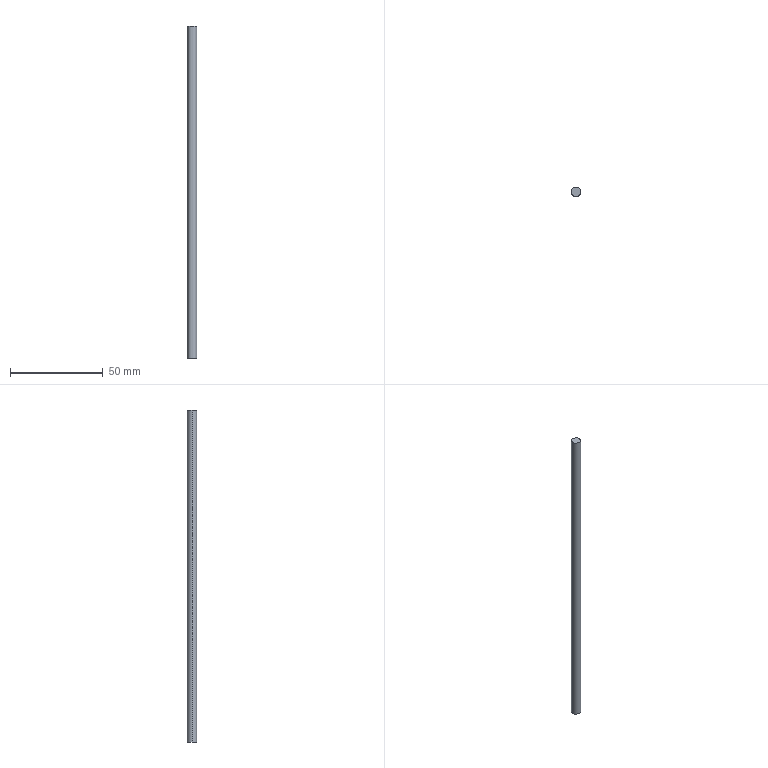Part | SolidWorks | features Extrusion 1 | 1 solid | 4 faces | box 5 x 5 x 178.5 mm | volume 3505 mm3 | cylinder 2 | plane 2 | commonest cylinder face diameters 5 x2
STEP:
#1=CARTESIAN_POINT('',(2.5,0.,178.5));
#2=VERTEX_POINT('',#1);
#3=CARTESIAN_POINT('',(-2.5,0.,178.5));
#4=VERTEX_POINT('',#3);
#5=CARTESIAN_POINT('',(0.,0.,178.5));
#6=DIRECTION('',(0.,0.,1.));
#7=DIRECTION('',(1.,0.,0.));
#8=AXIS2_PLACEMENT_3D('',#5,#6,#7);
#9=CIRCLE('',#8,2.5);
#10=EDGE_CURVE('',#2,#4,#9,.T.);
#11=ORIENTED_EDGE('',*,*,#10,.F.);
#12=CARTESIAN_POINT('',(2.5,0.,0.));
#13=VERTEX_POINT('',#12);
#14=CARTESIAN_POINT('',(2.5,0.,178.5));
#15=DIRECTION('',(0.,0.,-1.));
#16=VECTOR('',#15,1000.);
#17=LINE('',#14,#16);
#18=EDGE_CURVE('',#2,#13,#17,.T.);
#19=ORIENTED_EDGE('',*,*,#18,.T.);
#20=CARTESIAN_POINT('',(-2.5,0.,0.));
#21=VERTEX_POINT('',#20);
#22=CARTESIAN_POINT('',(0.,0.,0.));
#23=DIRECTION('',(0.,0.,1.));
#24=DIRECTION('',(1.,0.,0.));
#25=AXIS2_PLACEMENT_3D('',#22,#23,#24);
#26=CIRCLE('',#25,2.5);
#27=EDGE_CURVE('',#13,#21,#26,.T.);
#28=ORIENTED_EDGE('',*,*,#27,.T.);
#29=CARTESIAN_POINT('',(-2.5,0.,178.5));
#30=DIRECTION('',(0.,0.,-1.));
#31=VECTOR('',#30,1000.);
#32=LINE('',#29,#31);
#33=EDGE_CURVE('',#4,#21,#32,.T.);
#34=ORIENTED_EDGE('',*,*,#33,.F.);
#35=EDGE_LOOP('',(#11,#19,#28,#34));
#36=FACE_OUTER_BOUND('',#35,.T.);
#37=CARTESIAN_POINT('',(0.,0.,178.5));
#38=DIRECTION('',(0.,0.,-1.));
#39=DIRECTION('',(-1.,0.,0.));
#40=AXIS2_PLACEMENT_3D('',#37,#38,#39);
#41=CYLINDRICAL_SURFACE('',#40,2.5);
#42=ADVANCED_FACE('',(#36),#41,.T.);
#43=ORIENTED_EDGE('',*,*,#18,.F.);
#44=CARTESIAN_POINT('',(0.,0.,178.5));
#45=DIRECTION('',(0.,0.,1.));
#46=DIRECTION('',(1.,0.,0.));
#47=AXIS2_PLACEMENT_3D('',#44,#45,#46);
#48=CIRCLE('',#47,2.5);
#49=EDGE_CURVE('',#4,#2,#48,.T.);
#50=ORIENTED_EDGE('',*,*,#49,.F.);
#51=ORIENTED_EDGE('',*,*,#33,.T.);
#52=CARTESIAN_POINT('',(0.,0.,0.));
#53=DIRECTION('',(0.,0.,1.));
#54=DIRECTION('',(1.,0.,0.));
#55=AXIS2_PLACEMENT_3D('',#52,#53,#54);
#56=CIRCLE('',#55,2.5);
#57=EDGE_CURVE('',#21,#13,#56,.T.);
#58=ORIENTED_EDGE('',*,*,#57,.T.);
#59=EDGE_LOOP('',(#43,#50,#51,#58));
#60=FACE_OUTER_BOUND('',#59,.T.);
#61=CARTESIAN_POINT('',(0.,0.,178.5));
#62=DIRECTION('',(0.,0.,-1.));
#63=DIRECTION('',(-1.,0.,0.));
#64=AXIS2_PLACEMENT_3D('',#61,#62,#63);
#65=CYLINDRICAL_SURFACE('',#64,2.5);
#66=ADVANCED_FACE('',(#60),#65,.T.);
#67=ORIENTED_EDGE('',*,*,#49,.T.);
#68=ORIENTED_EDGE('',*,*,#10,.T.);
#69=EDGE_LOOP('',(#67,#68));
#70=FACE_OUTER_BOUND('',#69,.T.);
#71=CARTESIAN_POINT('',(0.,0.,178.5));
#72=DIRECTION('',(0.,0.,1.));
#73=DIRECTION('',(1.,0.,0.));
#74=AXIS2_PLACEMENT_3D('',#71,#72,#73);
#75=PLANE('',#74);
#76=ADVANCED_FACE('',(#70),#75,.T.);
#77=ORIENTED_EDGE('',*,*,#57,.F.);
#78=ORIENTED_EDGE('',*,*,#27,.F.);
#79=EDGE_LOOP('',(#77,#78));
#80=FACE_OUTER_BOUND('',#79,.T.);
#81=CARTESIAN_POINT('',(0.,0.,0.));
#82=DIRECTION('',(0.,0.,1.));
#83=DIRECTION('',(1.,0.,0.));
#84=AXIS2_PLACEMENT_3D('',#81,#82,#83);
#85=PLANE('',#84);
#86=ADVANCED_FACE('',(#80),#85,.F.);
#87=CLOSED_SHELL('',(#42,#66,#76,#86));
#88=MANIFOLD_SOLID_BREP('',#87);
#89=CARTESIAN_POINT('',(0.,0.,0.));
#90=DIRECTION('',(0.,0.,1.));
#91=DIRECTION('',(1.,0.,0.));
#92=AXIS2_PLACEMENT_3D('',#89,#90,#91);
#93=(LENGTH_UNIT()NAMED_UNIT(*)SI_UNIT(.MILLI.,.METRE.));
#94=UNCERTAINTY_MEASURE_WITH_UNIT(LENGTH_MEASURE(0.00001),#93,'','');
#95=(NAMED_UNIT(*)PLANE_ANGLE_UNIT()SI_UNIT($,.RADIAN.));
#96=(NAMED_UNIT(*)SI_UNIT($,.STERADIAN.)SOLID_ANGLE_UNIT());
#97=(GEOMETRIC_REPRESENTATION_CONTEXT(3)GLOBAL_UNCERTAINTY_ASSIGNED_CONTEXT((#94))GLOBAL_UNIT_ASSIGNED_CONTEXT((#93,#95,#96))REPRESENTATION_CONTEXT('',''));
#98=ADVANCED_BREP_SHAPE_REPRESENTATION('',(#88,#92),#97);